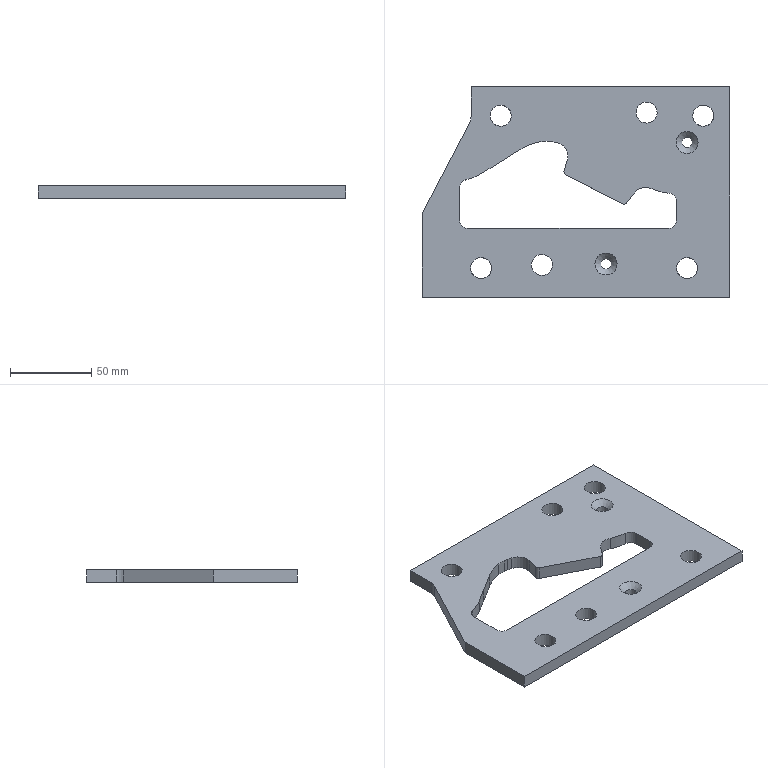Part | STEP file | gslz 2016.10.28-13_id766_x_t | 1 solid | 41 faces | box 190 x 130 x 8 mm | volume 142901 mm3 | cylinder 21 | plane 18 | cone 2 | commonest cylinder face diameters 13 x6 10 x4 4 x2 6.5 x2 18 x2 16 x1